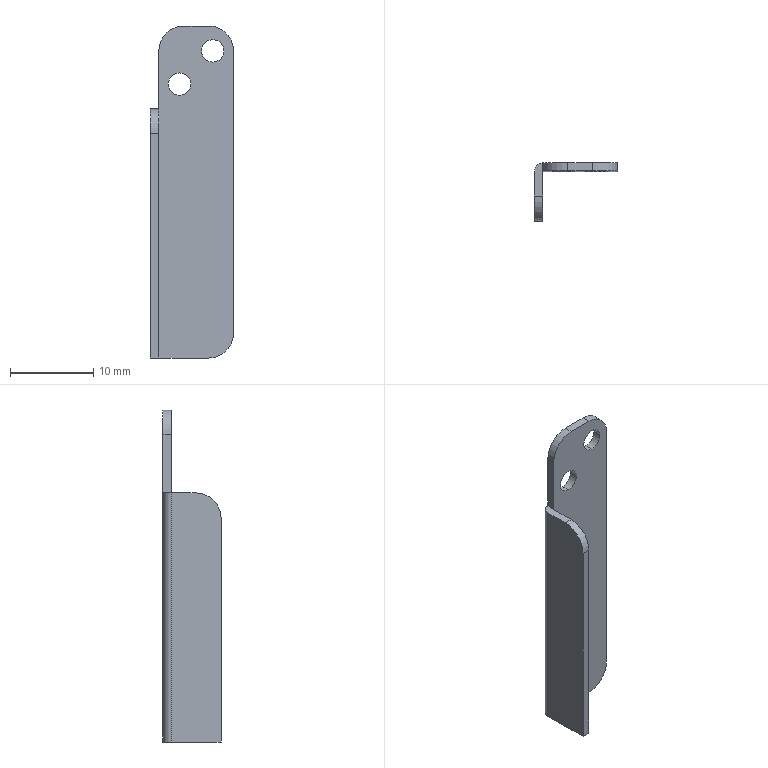Part | SolidWorks | features ICE 2, Fillet 1, FlatPattern 1, SMBaseFlange 1, SheetMetal 1 | 1 solid | 21 faces | box 10 x 7 x 40 mm | volume 544.385 mm3 | plane 12 | cylinder 9 | commonest cylinder face diameters 2.7 x4 6 x4 2 x1
STEP:
#1=CARTESIAN_POINT('',(3.5,6.,31.65));
#2=VERTEX_POINT('',#1);
#3=CARTESIAN_POINT('',(3.5,6.,34.35));
#4=VERTEX_POINT('',#3);
#5=CARTESIAN_POINT('',(3.5,6.,33.));
#6=DIRECTION('',(0.,1.,0.));
#7=DIRECTION('',(0.,0.,1.));
#8=AXIS2_PLACEMENT_3D('',#5,#6,#7);
#9=CIRCLE('',#8,1.35);
#10=EDGE_CURVE('',#2,#4,#9,.T.);
#11=ORIENTED_EDGE('',*,*,#10,.F.);
#12=CARTESIAN_POINT('',(3.5,7.,31.65));
#13=VERTEX_POINT('',#12);
#14=CARTESIAN_POINT('',(3.5,-3.,31.65));
#15=DIRECTION('',(0.,1.,0.));
#16=VECTOR('',#15,1000.);
#17=LINE('',#14,#16);
#18=EDGE_CURVE('',#2,#13,#17,.T.);
#19=ORIENTED_EDGE('',*,*,#18,.T.);
#20=CARTESIAN_POINT('',(3.5,7.,34.35));
#21=VERTEX_POINT('',#20);
#22=CARTESIAN_POINT('',(3.5,7.,33.));
#23=DIRECTION('',(0.,1.,0.));
#24=DIRECTION('',(0.,0.,1.));
#25=AXIS2_PLACEMENT_3D('',#22,#23,#24);
#26=CIRCLE('',#25,1.35);
#27=EDGE_CURVE('',#13,#21,#26,.T.);
#28=ORIENTED_EDGE('',*,*,#27,.T.);
#29=CARTESIAN_POINT('',(3.5,-3.,34.35));
#30=DIRECTION('',(0.,1.,0.));
#31=VECTOR('',#30,1000.);
#32=LINE('',#29,#31);
#33=EDGE_CURVE('',#4,#21,#32,.T.);
#34=ORIENTED_EDGE('',*,*,#33,.F.);
#35=EDGE_LOOP('',(#11,#19,#28,#34));
#36=FACE_OUTER_BOUND('',#35,.T.);
#37=CARTESIAN_POINT('',(3.5,-3.,33.));
#38=DIRECTION('',(0.,1.,0.));
#39=DIRECTION('',(0.,0.,1.));
#40=AXIS2_PLACEMENT_3D('',#37,#38,#39);
#41=CYLINDRICAL_SURFACE('',#40,1.35);
#42=ADVANCED_FACE('',(#36),#41,.F.);
#43=CARTESIAN_POINT('',(7.5,6.,35.65));
#44=VERTEX_POINT('',#43);
#45=CARTESIAN_POINT('',(7.5,6.,38.35));
#46=VERTEX_POINT('',#45);
#47=CARTESIAN_POINT('',(7.5,6.,37.));
#48=DIRECTION('',(0.,1.,0.));
#49=DIRECTION('',(0.,0.,1.));
#50=AXIS2_PLACEMENT_3D('',#47,#48,#49);
#51=CIRCLE('',#50,1.35);
#52=EDGE_CURVE('',#44,#46,#51,.T.);
#53=ORIENTED_EDGE('',*,*,#52,.F.);
#54=CARTESIAN_POINT('',(7.5,7.,35.65));
#55=VERTEX_POINT('',#54);
#56=CARTESIAN_POINT('',(7.5,-3.,35.65));
#57=DIRECTION('',(0.,1.,0.));
#58=VECTOR('',#57,1000.);
#59=LINE('',#56,#58);
#60=EDGE_CURVE('',#44,#55,#59,.T.);
#61=ORIENTED_EDGE('',*,*,#60,.T.);
#62=CARTESIAN_POINT('',(7.5,7.,38.35));
#63=VERTEX_POINT('',#62);
#64=CARTESIAN_POINT('',(7.5,7.,37.));
#65=DIRECTION('',(0.,1.,0.));
#66=DIRECTION('',(0.,0.,1.));
#67=AXIS2_PLACEMENT_3D('',#64,#65,#66);
#68=CIRCLE('',#67,1.35);
#69=EDGE_CURVE('',#55,#63,#68,.T.);
#70=ORIENTED_EDGE('',*,*,#69,.T.);
#71=CARTESIAN_POINT('',(7.5,-3.,38.35));
#72=DIRECTION('',(0.,1.,0.));
#73=VECTOR('',#72,1000.);
#74=LINE('',#71,#73);
#75=EDGE_CURVE('',#46,#63,#74,.T.);
#76=ORIENTED_EDGE('',*,*,#75,.F.);
#77=EDGE_LOOP('',(#53,#61,#70,#76));
#78=FACE_OUTER_BOUND('',#77,.T.);
#79=CARTESIAN_POINT('',(7.5,-3.,37.));
#80=DIRECTION('',(0.,1.,0.));
#81=DIRECTION('',(0.,0.,1.));
#82=AXIS2_PLACEMENT_3D('',#79,#80,#81);
#83=CYLINDRICAL_SURFACE('',#82,1.35);
#84=ADVANCED_FACE('',(#78),#83,.F.);
#85=CARTESIAN_POINT('',(4.,6.,40.));
#86=VERTEX_POINT('',#85);
#87=CARTESIAN_POINT('',(7.,6.,40.));
#88=VERTEX_POINT('',#87);
#89=CARTESIAN_POINT('',(0.,6.,40.));
#90=DIRECTION('',(1.,0.,0.));
#91=VECTOR('',#90,1000.);
#92=LINE('',#89,#91);
#93=EDGE_CURVE('',#86,#88,#92,.T.);
#94=ORIENTED_EDGE('',*,*,#93,.T.);
#95=CARTESIAN_POINT('',(7.,7.,40.));
#96=VERTEX_POINT('',#95);
#97=CARTESIAN_POINT('',(7.,6.,40.));
#98=DIRECTION('',(0.,1.,0.));
#99=VECTOR('',#98,1000.);
#100=LINE('',#97,#99);
#101=EDGE_CURVE('',#88,#96,#100,.T.);
#102=ORIENTED_EDGE('',*,*,#101,.T.);
#103=CARTESIAN_POINT('',(4.,7.,40.));
#104=VERTEX_POINT('',#103);
#105=CARTESIAN_POINT('',(0.,7.,40.));
#106=DIRECTION('',(1.,0.,0.));
#107=VECTOR('',#106,1000.);
#108=LINE('',#105,#107);
#109=EDGE_CURVE('',#104,#96,#108,.T.);
#110=ORIENTED_EDGE('',*,*,#109,.F.);
#111=CARTESIAN_POINT('',(4.,6.,40.));
#112=DIRECTION('',(0.,-1.,0.));
#113=VECTOR('',#112,1000.);
#114=LINE('',#111,#113);
#115=EDGE_CURVE('',#104,#86,#114,.T.);
#116=ORIENTED_EDGE('',*,*,#115,.T.);
#117=EDGE_LOOP('',(#94,#102,#110,#116));
#118=FACE_OUTER_BOUND('',#117,.T.);
#119=CARTESIAN_POINT('',(1.,6.,40.));
#120=DIRECTION('',(0.,0.,1.));
#121=DIRECTION('',(1.,0.,0.));
#122=AXIS2_PLACEMENT_3D('',#119,#120,#121);
#123=PLANE('',#122);
#124=ADVANCED_FACE('',(#118),#123,.T.);
#125=CARTESIAN_POINT('',(1.,6.,0.));
#126=VERTEX_POINT('',#125);
#127=CARTESIAN_POINT('',(0.,6.,0.));
#128=VERTEX_POINT('',#127);
#129=CARTESIAN_POINT('',(1.,6.,0.));
#130=DIRECTION('',(-1.,0.,0.));
#131=VECTOR('',#130,1000.);
#132=LINE('',#129,#131);
#133=EDGE_CURVE('',#126,#128,#132,.T.);
#134=ORIENTED_EDGE('',*,*,#133,.F.);
#135=CARTESIAN_POINT('',(1.,0.,0.));
#136=VERTEX_POINT('',#135);
#137=CARTESIAN_POINT('',(1.,0.,0.));
#138=DIRECTION('',(0.,1.,0.));
#139=VECTOR('',#138,1000.);
#140=LINE('',#137,#139);
#141=EDGE_CURVE('',#136,#126,#140,.T.);
#142=ORIENTED_EDGE('',*,*,#141,.F.);
#143=CARTESIAN_POINT('',(0.,0.,0.));
#144=VERTEX_POINT('',#143);
#145=CARTESIAN_POINT('',(1.,0.,0.));
#146=DIRECTION('',(-1.,0.,0.));
#147=VECTOR('',#146,1000.);
#148=LINE('',#145,#147);
#149=EDGE_CURVE('',#136,#144,#148,.T.);
#150=ORIENTED_EDGE('',*,*,#149,.T.);
#151=CARTESIAN_POINT('',(0.,0.,0.));
#152=DIRECTION('',(0.,1.,0.));
#153=VECTOR('',#152,1000.);
#154=LINE('',#151,#153);
#155=EDGE_CURVE('',#144,#128,#154,.T.);
#156=ORIENTED_EDGE('',*,*,#155,.T.);
#157=EDGE_LOOP('',(#134,#142,#150,#156));
#158=FACE_OUTER_BOUND('',#157,.T.);
#159=CARTESIAN_POINT('',(1.,6.,0.));
#160=DIRECTION('',(0.,0.,-1.));
#161=DIRECTION('',(-1.,0.,0.));
#162=AXIS2_PLACEMENT_3D('',#159,#160,#161);
#163=PLANE('',#162);
#164=ADVANCED_FACE('',(#158),#163,.T.);
#165=CARTESIAN_POINT('',(1.,7.,0.));
#166=VERTEX_POINT('',#165);
#167=CARTESIAN_POINT('',(1.,6.,0.));
#168=DIRECTION('',(0.,1.,0.));
#169=VECTOR('',#168,1000.);
#170=LINE('',#167,#169);
#171=EDGE_CURVE('',#126,#166,#170,.T.);
#172=ORIENTED_EDGE('',*,*,#171,.F.);
#173=ORIENTED_EDGE('',*,*,#133,.T.);
#174=CARTESIAN_POINT('',(1.,6.,0.));
#175=DIRECTION('',(0.,0.,-1.));
#176=DIRECTION('',(1.,0.,0.));
#177=AXIS2_PLACEMENT_3D('',#174,#175,#176);
#178=CIRCLE('',#177,1.);
#179=EDGE_CURVE('',#128,#166,#178,.T.);
#180=ORIENTED_EDGE('',*,*,#179,.T.);
#181=EDGE_LOOP('',(#172,#173,#180));
#182=FACE_OUTER_BOUND('',#181,.T.);
#183=CARTESIAN_POINT('',(1.,6.,0.));
#184=DIRECTION('',(0.,0.,-1.));
#185=DIRECTION('',(-1.,0.,0.));
#186=AXIS2_PLACEMENT_3D('',#183,#184,#185);
#187=PLANE('',#186);
#188=ADVANCED_FACE('',(#182),#187,.T.);
#189=CARTESIAN_POINT('',(3.5,6.,33.));
#190=DIRECTION('',(0.,1.,0.));
#191=DIRECTION('',(0.,0.,1.));
#192=AXIS2_PLACEMENT_3D('',#189,#190,#191);
#193=CIRCLE('',#192,1.35);
#194=EDGE_CURVE('',#4,#2,#193,.T.);
#195=ORIENTED_EDGE('',*,*,#194,.T.);
#196=ORIENTED_EDGE('',*,*,#10,.T.);
#197=EDGE_LOOP('',(#195,#196));
#198=FACE_BOUND('',#197,.T.);
#199=CARTESIAN_POINT('',(7.5,6.,37.));
#200=DIRECTION('',(0.,1.,0.));
#201=DIRECTION('',(0.,0.,1.));
#202=AXIS2_PLACEMENT_3D('',#199,#200,#201);
#203=CIRCLE('',#202,1.35);
#204=EDGE_CURVE('',#46,#44,#203,.T.);
#205=ORIENTED_EDGE('',*,*,#204,.T.);
#206=ORIENTED_EDGE('',*,*,#52,.T.);
#207=EDGE_LOOP('',(#205,#206));
#208=FACE_BOUND('',#207,.T.);
#209=CARTESIAN_POINT('',(7.,6.,0.));
#210=VERTEX_POINT('',#209);
#211=CARTESIAN_POINT('',(0.,6.,0.));
#212=DIRECTION('',(1.,0.,0.));
#213=VECTOR('',#212,1000.);
#214=LINE('',#211,#213);
#215=EDGE_CURVE('',#126,#210,#214,.T.);
#216=ORIENTED_EDGE('',*,*,#215,.T.);
#217=CARTESIAN_POINT('',(10.,6.,3.));
#218=VERTEX_POINT('',#217);
#219=CARTESIAN_POINT('',(7.,6.,3.));
#220=DIRECTION('',(0.,-1.,0.));
#221=DIRECTION('',(0.,0.,1.));
#222=AXIS2_PLACEMENT_3D('',#219,#220,#221);
#223=CIRCLE('',#222,3.);
#224=EDGE_CURVE('',#210,#218,#223,.T.);
#225=ORIENTED_EDGE('',*,*,#224,.T.);
#226=CARTESIAN_POINT('',(10.,6.,37.));
#227=VERTEX_POINT('',#226);
#228=CARTESIAN_POINT('',(10.,6.,40.));
#229=DIRECTION('',(0.,0.,-1.));
#230=VECTOR('',#229,1000.);
#231=LINE('',#228,#230);
#232=EDGE_CURVE('',#227,#218,#231,.T.);
#233=ORIENTED_EDGE('',*,*,#232,.F.);
#234=CARTESIAN_POINT('',(7.,6.,37.));
#235=DIRECTION('',(0.,-1.,0.));
#236=DIRECTION('',(0.,0.,1.));
#237=AXIS2_PLACEMENT_3D('',#234,#235,#236);
#238=CIRCLE('',#237,3.);
#239=EDGE_CURVE('',#227,#88,#238,.T.);
#240=ORIENTED_EDGE('',*,*,#239,.T.);
#241=ORIENTED_EDGE('',*,*,#93,.F.);
#242=CARTESIAN_POINT('',(1.,6.,37.));
#243=VERTEX_POINT('',#242);
#244=CARTESIAN_POINT('',(4.,6.,37.));
#245=DIRECTION('',(0.,-1.,0.));
#246=DIRECTION('',(0.,0.,1.));
#247=AXIS2_PLACEMENT_3D('',#244,#245,#246);
#248=CIRCLE('',#247,3.);
#249=EDGE_CURVE('',#86,#243,#248,.T.);
#250=ORIENTED_EDGE('',*,*,#249,.T.);
#251=CARTESIAN_POINT('',(1.,6.,30.));
#252=VERTEX_POINT('',#251);
#253=CARTESIAN_POINT('',(1.,6.,40.));
#254=DIRECTION('',(0.,0.,-1.));
#255=VECTOR('',#254,1000.);
#256=LINE('',#253,#255);
#257=EDGE_CURVE('',#243,#252,#256,.T.);
#258=ORIENTED_EDGE('',*,*,#257,.T.);
#259=CARTESIAN_POINT('',(1.,6.,40.));
#260=DIRECTION('',(0.,0.,-1.));
#261=VECTOR('',#260,1000.);
#262=LINE('',#259,#261);
#263=EDGE_CURVE('',#252,#126,#262,.T.);
#264=ORIENTED_EDGE('',*,*,#263,.T.);
#265=EDGE_LOOP('',(#216,#225,#233,#240,#241,#250,#258,#264));
#266=FACE_OUTER_BOUND('',#265,.T.);
#267=CARTESIAN_POINT('',(0.,6.,40.));
#268=DIRECTION('',(0.,1.,0.));
#269=DIRECTION('',(0.,0.,1.));
#270=AXIS2_PLACEMENT_3D('',#267,#268,#269);
#271=PLANE('',#270);
#272=ADVANCED_FACE('',(#198,#208,#266),#271,.F.);
#273=ORIENTED_EDGE('',*,*,#232,.T.);
#274=CARTESIAN_POINT('',(10.,7.,3.));
#275=VERTEX_POINT('',#274);
#276=CARTESIAN_POINT('',(10.,7.,3.));
#277=DIRECTION('',(0.,1.,0.));
#278=VECTOR('',#277,1000.);
#279=LINE('',#276,#278);
#280=EDGE_CURVE('',#218,#275,#279,.T.);
#281=ORIENTED_EDGE('',*,*,#280,.T.);
#282=CARTESIAN_POINT('',(10.,7.,37.));
#283=VERTEX_POINT('',#282);
#284=CARTESIAN_POINT('',(10.,7.,40.));
#285=DIRECTION('',(0.,0.,-1.));
#286=VECTOR('',#285,1000.);
#287=LINE('',#284,#286);
#288=EDGE_CURVE('',#283,#275,#287,.T.);
#289=ORIENTED_EDGE('',*,*,#288,.F.);
#290=CARTESIAN_POINT('',(10.,7.,37.));
#291=DIRECTION('',(0.,-1.,0.));
#292=VECTOR('',#291,1000.);
#293=LINE('',#290,#292);
#294=EDGE_CURVE('',#283,#227,#293,.T.);
#295=ORIENTED_EDGE('',*,*,#294,.T.);
#296=EDGE_LOOP('',(#273,#281,#289,#295));
#297=FACE_OUTER_BOUND('',#296,.T.);
#298=CARTESIAN_POINT('',(10.,7.,40.));
#299=DIRECTION('',(1.,0.,0.));
#300=DIRECTION('',(0.,0.,-1.));
#301=AXIS2_PLACEMENT_3D('',#298,#299,#300);
#302=PLANE('',#301);
#303=ADVANCED_FACE('',(#297),#302,.T.);
#304=CARTESIAN_POINT('',(3.5,7.,33.));
#305=DIRECTION('',(0.,1.,0.));
#306=DIRECTION('',(0.,0.,1.));
#307=AXIS2_PLACEMENT_3D('',#304,#305,#306);
#308=CIRCLE('',#307,1.35);
#309=EDGE_CURVE('',#21,#13,#308,.T.);
#310=ORIENTED_EDGE('',*,*,#309,.F.);
#311=ORIENTED_EDGE('',*,*,#27,.F.);
#312=EDGE_LOOP('',(#310,#311));
#313=FACE_BOUND('',#312,.T.);
#314=CARTESIAN_POINT('',(7.5,7.,37.));
#315=DIRECTION('',(0.,1.,0.));
#316=DIRECTION('',(0.,0.,1.));
#317=AXIS2_PLACEMENT_3D('',#314,#315,#316);
#318=CIRCLE('',#317,1.35);
#319=EDGE_CURVE('',#63,#55,#318,.T.);
#320=ORIENTED_EDGE('',*,*,#319,.F.);
#321=ORIENTED_EDGE('',*,*,#69,.F.);
#322=EDGE_LOOP('',(#320,#321));
#323=FACE_BOUND('',#322,.T.);
#324=ORIENTED_EDGE('',*,*,#288,.T.);
#325=CARTESIAN_POINT('',(7.,7.,0.));
#326=VERTEX_POINT('',#325);
#327=CARTESIAN_POINT('',(7.,7.,3.));
#328=DIRECTION('',(0.,1.,0.));
#329=DIRECTION('',(0.,0.,1.));
#330=AXIS2_PLACEMENT_3D('',#327,#328,#329);
#331=CIRCLE('',#330,3.);
#332=EDGE_CURVE('',#275,#326,#331,.T.);
#333=ORIENTED_EDGE('',*,*,#332,.T.);
#334=CARTESIAN_POINT('',(0.,7.,0.));
#335=DIRECTION('',(1.,0.,0.));
#336=VECTOR('',#335,1000.);
#337=LINE('',#334,#336);
#338=EDGE_CURVE('',#166,#326,#337,.T.);
#339=ORIENTED_EDGE('',*,*,#338,.F.);
#340=CARTESIAN_POINT('',(1.,7.,30.));
#341=VERTEX_POINT('',#340);
#342=CARTESIAN_POINT('',(1.,7.,40.));
#343=DIRECTION('',(0.,0.,-1.));
#344=VECTOR('',#343,1000.);
#345=LINE('',#342,#344);
#346=EDGE_CURVE('',#341,#166,#345,.T.);
#347=ORIENTED_EDGE('',*,*,#346,.F.);
#348=CARTESIAN_POINT('',(1.,7.,37.));
#349=VERTEX_POINT('',#348);
#350=CARTESIAN_POINT('',(1.,7.,40.));
#351=DIRECTION('',(0.,0.,-1.));
#352=VECTOR('',#351,1000.);
#353=LINE('',#350,#352);
#354=EDGE_CURVE('',#349,#341,#353,.T.);
#355=ORIENTED_EDGE('',*,*,#354,.F.);
#356=CARTESIAN_POINT('',(4.,7.,37.));
#357=DIRECTION('',(0.,1.,0.));
#358=DIRECTION('',(0.,0.,1.));
#359=AXIS2_PLACEMENT_3D('',#356,#357,#358);
#360=CIRCLE('',#359,3.);
#361=EDGE_CURVE('',#349,#104,#360,.T.);
#362=ORIENTED_EDGE('',*,*,#361,.T.);
#363=ORIENTED_EDGE('',*,*,#109,.T.);
#364=CARTESIAN_POINT('',(7.,7.,37.));
#365=DIRECTION('',(0.,1.,0.));
#366=DIRECTION('',(0.,0.,1.));
#367=AXIS2_PLACEMENT_3D('',#364,#365,#366);
#368=CIRCLE('',#367,3.);
#369=EDGE_CURVE('',#96,#283,#368,.T.);
#370=ORIENTED_EDGE('',*,*,#369,.T.);
#371=EDGE_LOOP('',(#324,#333,#339,#347,#355,#362,#363,#370));
#372=FACE_OUTER_BOUND('',#371,.T.);
#373=CARTESIAN_POINT('',(0.,7.,40.));
#374=DIRECTION('',(0.,1.,0.));
#375=DIRECTION('',(0.,0.,1.));
#376=AXIS2_PLACEMENT_3D('',#373,#374,#375);
#377=PLANE('',#376);
#378=ADVANCED_FACE('',(#313,#323,#372),#377,.T.);
#379=CARTESIAN_POINT('',(0.,6.,30.));
#380=VERTEX_POINT('',#379);
#381=CARTESIAN_POINT('',(1.,6.,30.));
#382=DIRECTION('',(0.,0.,1.));
#383=DIRECTION('',(-1.,0.,0.));
#384=AXIS2_PLACEMENT_3D('',#381,#382,#383);
#385=CIRCLE('',#384,1.);
#386=EDGE_CURVE('',#341,#380,#385,.T.);
#387=ORIENTED_EDGE('',*,*,#386,.F.);
#388=ORIENTED_EDGE('',*,*,#346,.T.);
#389=ORIENTED_EDGE('',*,*,#179,.F.);
#390=CARTESIAN_POINT('',(0.,6.,40.));
#391=DIRECTION('',(0.,0.,-1.));
#392=VECTOR('',#391,1000.);
#393=LINE('',#390,#392);
#394=EDGE_CURVE('',#380,#128,#393,.T.);
#395=ORIENTED_EDGE('',*,*,#394,.F.);
#396=EDGE_LOOP('',(#387,#388,#389,#395));
#397=FACE_OUTER_BOUND('',#396,.T.);
#398=CARTESIAN_POINT('',(1.,6.,40.));
#399=DIRECTION('',(0.,0.,-1.));
#400=DIRECTION('',(-1.,0.,0.));
#401=AXIS2_PLACEMENT_3D('',#398,#399,#400);
#402=CYLINDRICAL_SURFACE('',#401,1.);
#403=ADVANCED_FACE('',(#397),#402,.T.);
#404=CARTESIAN_POINT('',(0.,0.,27.));
#405=VERTEX_POINT('',#404);
#406=CARTESIAN_POINT('',(0.,0.,40.));
#407=DIRECTION('',(0.,0.,-1.));
#408=VECTOR('',#407,1000.);
#409=LINE('',#406,#408);
#410=EDGE_CURVE('',#405,#144,#409,.T.);
#411=ORIENTED_EDGE('',*,*,#410,.F.);
#412=CARTESIAN_POINT('',(0.,3.,30.));
#413=VERTEX_POINT('',#412);
#414=CARTESIAN_POINT('',(0.,3.,27.));
#415=DIRECTION('',(-1.,0.,0.));
#416=DIRECTION('',(0.,0.,1.));
#417=AXIS2_PLACEMENT_3D('',#414,#415,#416);
#418=CIRCLE('',#417,3.);
#419=EDGE_CURVE('',#405,#413,#418,.T.);
#420=ORIENTED_EDGE('',*,*,#419,.T.);
#421=CARTESIAN_POINT('',(0.,7.,30.));
#422=DIRECTION('',(0.,-1.,0.));
#423=VECTOR('',#422,1000.);
#424=LINE('',#421,#423);
#425=EDGE_CURVE('',#380,#413,#424,.T.);
#426=ORIENTED_EDGE('',*,*,#425,.F.);
#427=ORIENTED_EDGE('',*,*,#394,.T.);
#428=ORIENTED_EDGE('',*,*,#155,.F.);
#429=EDGE_LOOP('',(#411,#420,#426,#427,#428));
#430=FACE_OUTER_BOUND('',#429,.T.);
#431=CARTESIAN_POINT('',(0.,0.,40.));
#432=DIRECTION('',(-1.,0.,0.));
#433=DIRECTION('',(0.,0.,1.));
#434=AXIS2_PLACEMENT_3D('',#431,#432,#433);
#435=PLANE('',#434);
#436=ADVANCED_FACE('',(#430),#435,.T.);
#437=CARTESIAN_POINT('',(1.,0.,27.));
#438=VERTEX_POINT('',#437);
#439=CARTESIAN_POINT('',(1.,0.,40.));
#440=DIRECTION('',(0.,0.,-1.));
#441=VECTOR('',#440,1000.);
#442=LINE('',#439,#441);
#443=EDGE_CURVE('',#438,#136,#442,.T.);
#444=ORIENTED_EDGE('',*,*,#443,.F.);
#445=CARTESIAN_POINT('',(0.,0.,27.));
#446=DIRECTION('',(-1.,0.,0.));
#447=VECTOR('',#446,1000.);
#448=LINE('',#445,#447);
#449=EDGE_CURVE('',#438,#405,#448,.T.);
#450=ORIENTED_EDGE('',*,*,#449,.T.);
#451=ORIENTED_EDGE('',*,*,#410,.T.);
#452=ORIENTED_EDGE('',*,*,#149,.F.);
#453=EDGE_LOOP('',(#444,#450,#451,#452));
#454=FACE_OUTER_BOUND('',#453,.T.);
#455=CARTESIAN_POINT('',(1.,0.,40.));
#456=DIRECTION('',(0.,-1.,0.));
#457=DIRECTION('',(0.,0.,-1.));
#458=AXIS2_PLACEMENT_3D('',#455,#456,#457);
#459=PLANE('',#458);
#460=ADVANCED_FACE('',(#454),#459,.T.);
#461=CARTESIAN_POINT('',(1.,3.,30.));
#462=VERTEX_POINT('',#461);
#463=CARTESIAN_POINT('',(1.,7.,30.));
#464=DIRECTION('',(0.,-1.,0.));
#465=VECTOR('',#464,1000.);
#466=LINE('',#463,#465);
#467=EDGE_CURVE('',#252,#462,#466,.T.);
#468=ORIENTED_EDGE('',*,*,#467,.T.);
#469=CARTESIAN_POINT('',(1.,3.,27.));
#470=DIRECTION('',(1.,0.,0.));
#471=DIRECTION('',(0.,0.,1.));
#472=AXIS2_PLACEMENT_3D('',#469,#470,#471);
#473=CIRCLE('',#472,3.);
#474=EDGE_CURVE('',#462,#438,#473,.T.);
#475=ORIENTED_EDGE('',*,*,#474,.T.);
#476=ORIENTED_EDGE('',*,*,#443,.T.);
#477=ORIENTED_EDGE('',*,*,#141,.T.);
#478=ORIENTED_EDGE('',*,*,#263,.F.);
#479=EDGE_LOOP('',(#468,#475,#476,#477,#478));
#480=FACE_OUTER_BOUND('',#479,.T.);
#481=CARTESIAN_POINT('',(1.,0.,40.));
#482=DIRECTION('',(-1.,0.,0.));
#483=DIRECTION('',(0.,0.,1.));
#484=AXIS2_PLACEMENT_3D('',#481,#482,#483);
#485=PLANE('',#484);
#486=ADVANCED_FACE('',(#480),#485,.F.);
#487=ORIENTED_EDGE('',*,*,#338,.T.);
#488=CARTESIAN_POINT('',(7.,6.,0.));
#489=DIRECTION('',(0.,-1.,0.));
#490=VECTOR('',#489,1000.);
#491=LINE('',#488,#490);
#492=EDGE_CURVE('',#326,#210,#491,.T.);
#493=ORIENTED_EDGE('',*,*,#492,.T.);
#494=ORIENTED_EDGE('',*,*,#215,.F.);
#495=ORIENTED_EDGE('',*,*,#171,.T.);
#496=EDGE_LOOP('',(#487,#493,#494,#495));
#497=FACE_OUTER_BOUND('',#496,.T.);
#498=CARTESIAN_POINT('',(1.,6.,0.));
#499=DIRECTION('',(0.,0.,1.));
#500=DIRECTION('',(1.,0.,0.));
#501=AXIS2_PLACEMENT_3D('',#498,#499,#500);
#502=PLANE('',#501);
#503=ADVANCED_FACE('',(#497),#502,.F.);
#504=ORIENTED_EDGE('',*,*,#257,.F.);
#505=CARTESIAN_POINT('',(1.,7.,37.));
#506=DIRECTION('',(0.,1.,0.));
#507=VECTOR('',#506,1000.);
#508=LINE('',#505,#507);
#509=EDGE_CURVE('',#243,#349,#508,.T.);
#510=ORIENTED_EDGE('',*,*,#509,.T.);
#511=ORIENTED_EDGE('',*,*,#354,.T.);
#512=CARTESIAN_POINT('',(1.,7.,30.));
#513=DIRECTION('',(0.,-1.,0.));
#514=VECTOR('',#513,1000.);
#515=LINE('',#512,#514);
#516=EDGE_CURVE('',#341,#252,#515,.T.);
#517=ORIENTED_EDGE('',*,*,#516,.T.);
#518=EDGE_LOOP('',(#504,#510,#511,#517));
#519=FACE_OUTER_BOUND('',#518,.T.);
#520=CARTESIAN_POINT('',(1.,7.,40.));
#521=DIRECTION('',(1.,0.,0.));
#522=DIRECTION('',(0.,0.,-1.));
#523=AXIS2_PLACEMENT_3D('',#520,#521,#522);
#524=PLANE('',#523);
#525=ADVANCED_FACE('',(#519),#524,.F.);
#526=ORIENTED_EDGE('',*,*,#425,.T.);
#527=CARTESIAN_POINT('',(1.,3.,30.));
#528=DIRECTION('',(1.,0.,0.));
#529=VECTOR('',#528,1000.);
#530=LINE('',#527,#529);
#531=EDGE_CURVE('',#413,#462,#530,.T.);
#532=ORIENTED_EDGE('',*,*,#531,.T.);
#533=ORIENTED_EDGE('',*,*,#467,.F.);
#534=ORIENTED_EDGE('',*,*,#516,.F.);
#535=ORIENTED_EDGE('',*,*,#386,.T.);
#536=EDGE_LOOP('',(#526,#532,#533,#534,#535));
#537=FACE_OUTER_BOUND('',#536,.T.);
#538=CARTESIAN_POINT('',(0.,7.,30.));
#539=DIRECTION('',(0.,0.,-1.));
#540=DIRECTION('',(-1.,0.,0.));
#541=AXIS2_PLACEMENT_3D('',#538,#539,#540);
#542=PLANE('',#541);
#543=ADVANCED_FACE('',(#537),#542,.F.);
#544=ORIENTED_EDGE('',*,*,#60,.F.);
#545=ORIENTED_EDGE('',*,*,#204,.F.);
#546=ORIENTED_EDGE('',*,*,#75,.T.);
#547=ORIENTED_EDGE('',*,*,#319,.T.);
#548=EDGE_LOOP('',(#544,#545,#546,#547));
#549=FACE_OUTER_BOUND('',#548,.T.);
#550=CARTESIAN_POINT('',(7.5,-3.,37.));
#551=DIRECTION('',(0.,1.,0.));
#552=DIRECTION('',(0.,0.,1.));
#553=AXIS2_PLACEMENT_3D('',#550,#551,#552);
#554=CYLINDRICAL_SURFACE('',#553,1.35);
#555=ADVANCED_FACE('',(#549),#554,.F.);
#556=ORIENTED_EDGE('',*,*,#18,.F.);
#557=ORIENTED_EDGE('',*,*,#194,.F.);
#558=ORIENTED_EDGE('',*,*,#33,.T.);
#559=ORIENTED_EDGE('',*,*,#309,.T.);
#560=EDGE_LOOP('',(#556,#557,#558,#559));
#561=FACE_OUTER_BOUND('',#560,.T.);
#562=CARTESIAN_POINT('',(3.5,-3.,33.));
#563=DIRECTION('',(0.,1.,0.));
#564=DIRECTION('',(0.,0.,1.));
#565=AXIS2_PLACEMENT_3D('',#562,#563,#564);
#566=CYLINDRICAL_SURFACE('',#565,1.35);
#567=ADVANCED_FACE('',(#561),#566,.F.);
#568=ORIENTED_EDGE('',*,*,#419,.F.);
#569=ORIENTED_EDGE('',*,*,#449,.F.);
#570=ORIENTED_EDGE('',*,*,#474,.F.);
#571=ORIENTED_EDGE('',*,*,#531,.F.);
#572=EDGE_LOOP('',(#568,#569,#570,#571));
#573=FACE_OUTER_BOUND('',#572,.T.);
#574=CARTESIAN_POINT('',(0.,3.,27.));
#575=DIRECTION('',(-1.,0.,0.));
#576=DIRECTION('',(0.,0.,1.));
#577=AXIS2_PLACEMENT_3D('',#574,#575,#576);
#578=CYLINDRICAL_SURFACE('',#577,3.);
#579=ADVANCED_FACE('',(#573),#578,.T.);
#580=ORIENTED_EDGE('',*,*,#332,.F.);
#581=ORIENTED_EDGE('',*,*,#280,.F.);
#582=ORIENTED_EDGE('',*,*,#224,.F.);
#583=ORIENTED_EDGE('',*,*,#492,.F.);
#584=EDGE_LOOP('',(#580,#581,#582,#583));
#585=FACE_OUTER_BOUND('',#584,.T.);
#586=CARTESIAN_POINT('',(7.,6.,3.));
#587=DIRECTION('',(0.,1.,0.));
#588=DIRECTION('',(0.,0.,1.));
#589=AXIS2_PLACEMENT_3D('',#586,#587,#588);
#590=CYLINDRICAL_SURFACE('',#589,3.);
#591=ADVANCED_FACE('',(#585),#590,.T.);
#592=ORIENTED_EDGE('',*,*,#369,.F.);
#593=ORIENTED_EDGE('',*,*,#101,.F.);
#594=ORIENTED_EDGE('',*,*,#239,.F.);
#595=ORIENTED_EDGE('',*,*,#294,.F.);
#596=EDGE_LOOP('',(#592,#593,#594,#595));
#597=FACE_OUTER_BOUND('',#596,.T.);
#598=CARTESIAN_POINT('',(7.,7.,37.));
#599=DIRECTION('',(0.,-1.,0.));
#600=DIRECTION('',(0.,0.,-1.));
#601=AXIS2_PLACEMENT_3D('',#598,#599,#600);
#602=CYLINDRICAL_SURFACE('',#601,3.);
#603=ADVANCED_FACE('',(#597),#602,.T.);
#604=ORIENTED_EDGE('',*,*,#249,.F.);
#605=ORIENTED_EDGE('',*,*,#115,.F.);
#606=ORIENTED_EDGE('',*,*,#361,.F.);
#607=ORIENTED_EDGE('',*,*,#509,.F.);
#608=EDGE_LOOP('',(#604,#605,#606,#607));
#609=FACE_OUTER_BOUND('',#608,.T.);
#610=CARTESIAN_POINT('',(4.,7.,37.));
#611=DIRECTION('',(0.,-1.,0.));
#612=DIRECTION('',(0.,0.,-1.));
#613=AXIS2_PLACEMENT_3D('',#610,#611,#612);
#614=CYLINDRICAL_SURFACE('',#613,3.);
#615=ADVANCED_FACE('',(#609),#614,.T.);
#616=CLOSED_SHELL('',(#42,#84,#124,#164,#188,#272,#303,#378,#403,#436,#460,#486,#503,#525,#543,#555,#567,#579,#591,#603,#615));
#617=MANIFOLD_SOLID_BREP('',#616);
#618=CARTESIAN_POINT('',(0.,0.,0.));
#619=DIRECTION('',(0.,0.,1.));
#620=DIRECTION('',(1.,0.,0.));
#621=AXIS2_PLACEMENT_3D('',#618,#619,#620);
#622=(LENGTH_UNIT()NAMED_UNIT(*)SI_UNIT(.MILLI.,.METRE.));
#623=UNCERTAINTY_MEASURE_WITH_UNIT(LENGTH_MEASURE(0.00001),#622,'','');
#624=(NAMED_UNIT(*)PLANE_ANGLE_UNIT()SI_UNIT($,.RADIAN.));
#625=(NAMED_UNIT(*)SI_UNIT($,.STERADIAN.)SOLID_ANGLE_UNIT());
#626=(GEOMETRIC_REPRESENTATION_CONTEXT(3)GLOBAL_UNCERTAINTY_ASSIGNED_CONTEXT((#623))GLOBAL_UNIT_ASSIGNED_CONTEXT((#622,#624,#625))REPRESENTATION_CONTEXT('',''));
#627=ADVANCED_BREP_SHAPE_REPRESENTATION('',(#617,#621),#626);